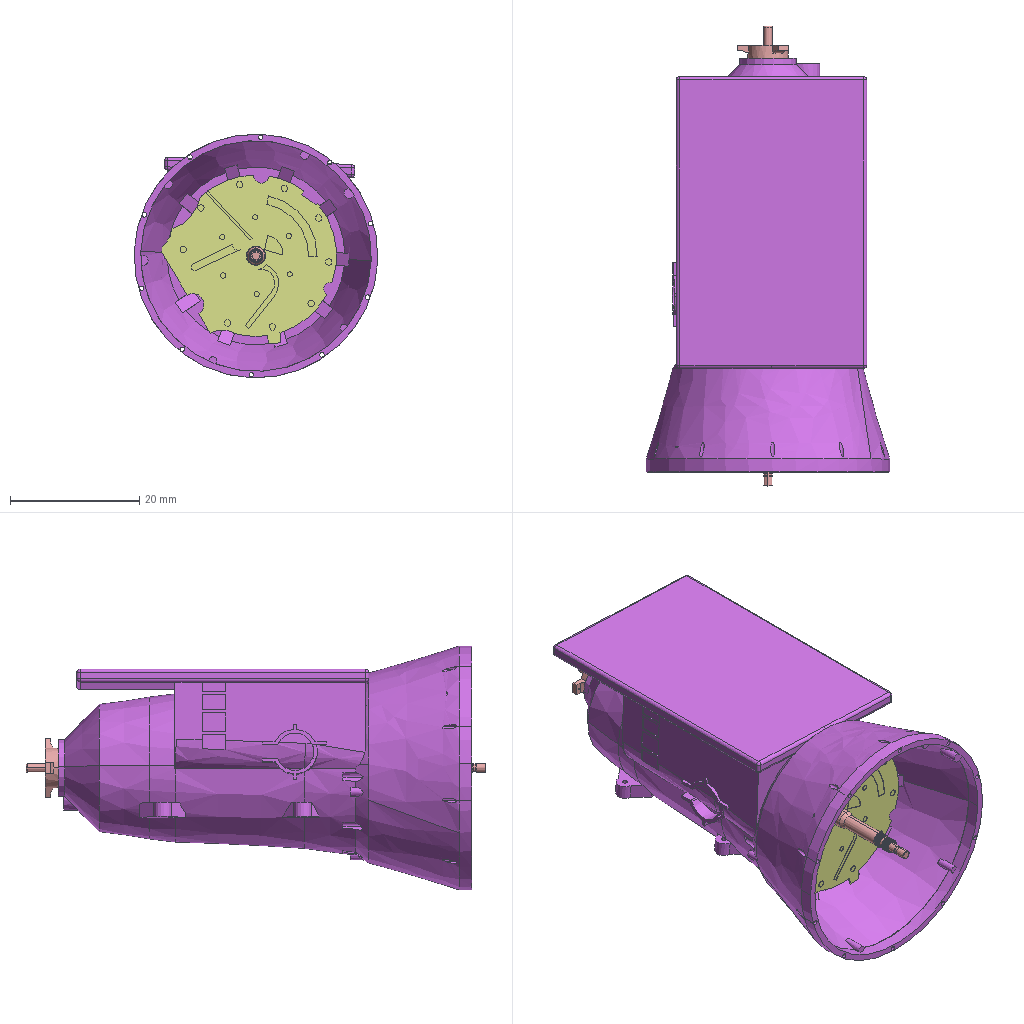Assembly | SolidWorks | 12 different items | 12 placed | box 38 x 71 x 38 mm
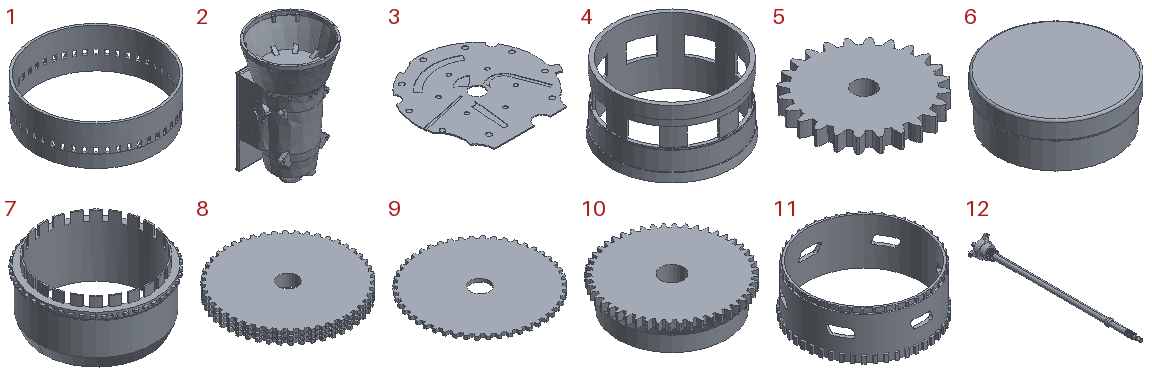Parts list (item | quantity | size | volume | features):
1 | x1 | 18.7 x 18.7 x 6 mm | 97.096 mm3 | features ICE 3, CirPattern 1, Extrusion 1
2 | x1 | 37.751 x 37.751 x 64.09 mm | 13251 mm3 | features ICE 18, Blend 7, DelFace 4, Fillet 4, CirPattern 2, MirrorPattern 2, BlendCut 1, Extrusion 1, Rib 1, Shell 1
3 | x1 | 26.026 x 24.754 x 0.2 mm | 92.065 mm3 | features ICE 4, Extrusion 1
4 | x1 | 19.3 x 19.3 x 10.5 mm | 297.419 mm3 | features ICE 7, Blend 1, CirPattern 1
5 | x1 | 16.941 x 16.941 x 3.8 mm | 406.625 mm3 | features ICE 2, Blend 1, CirPattern 1, Cut 1, Extrusion 1, Fillet 1
6 | x1 | 18 x 18 x 6.8 mm | 1583 mm3 | features Cut 1, Extrusion 1, Fillet 1, ICE 1
7 | x1 | 19.179 x 19.179 x 9.6 mm | 364.987 mm3 | features ICE 5, CirPattern 2, Blend 1, Extrusion 1, Fillet 1
8 | x1 | 19.259 x 19.259 x 1.9 mm | 502.853 mm3 | features ICE 7, CirPattern 3, Cut 1, Extrusion 1
9 | x1 | 19.259 x 19.259 x 0.5 mm | 134.631 mm3 | features CirPattern 1, Cut 1, Extrusion 1, ICE 1
10 | x1 | 16.296 x 16.296 x 4 mm | 653.065 mm3 | features ICE 2, Blend 1, CirPattern 1, Cut 1, Extrusion 1
11 | x1 | 18.565 x 18.565 x 7 mm | 181.204 mm3 | features ICE 4, CirPattern 3, Extrusion 1
12 | x1 | 7.952 x 71.26 x 9.182 mm | 329.036 mm3 | features ICE 5, CirPattern 4, Fillet 3, Cut 2, Revolution 2
Mates (type | each side: item.copy, entity, surface, feature):
Concentric | 12.1 face cylinder Revolve2 | 5.1 face cylinder Cut-Extrude1
Coincident | 12.1 face plane Boss-Extrude3 | 5.1 face plane Boss-Extrude3
Concentric | 12.1 face cylinder Revolve2 | 6.1 face cylinder Cut-Extrude1
Concentric | 12.1 face cylinder Revolve2 | 7.1 face cylinder Cut-Extrude2
Coincident | 6.1 face plane Boss-Extrude2 | 7.1 face plane Loft1
Concentric | 12.1 face cylinder Revolve2 | 8.1 face cylinder Cut-Extrude1
Coincident | 7.1 face plane CirPattern2 | 8.1 face plane Boss-Extrude7
Concentric | 12.1 face cylinder Revolve2 | 9.1 face cylinder Cut-Extrude1
Coincident | 8.1 face plane Boss-Extrude1 | 9.1 face plane Boss-Extrude1
Concentric | 12.1 face cylinder Revolve2 | 10.1 face cylinder Cut-Extrude1
Coincident | 9.1 face plane Boss-Extrude1 | 10.1 face plane Boss-Extrude2
Concentric | 12.1 face cylinder Revolve2 | 11.1 face cylinder Cut-Extrude1
Coincident | 10.1 face plane Boss-Extrude1 | 11.1 face plane Boss-Extrude1
Concentric | 12.1 face cylinder Revolve2 | 1.1 face cylinder Cut-Extrude1
Coincident | 11.1 face plane CirPattern2 | 1.1 face plane Cut-Extrude2 | 2 times
Concentric | 12.1 face cylinder Revolve2 | 4.1 face cylinder Cut-Extrude1
Coincident | 4.1 face plane Loft2 | 1.1 face plane Boss-Extrude2
Concentric | 12.1 face cylinder Revolve2 | 3.1 face cylinder Cut-Extrude1
Coincident | 12.1 face plane Revolve2 | 3.1 face plane Boss-Extrude2
GearDim | 8.1 face cylinder Boss-Extrude7 | 5.1 face cylinder Boss-Extrude1
GearDim | 9.1 face cylinder Boss-Extrude1 | 5.1 face cylinder Boss-Extrude1
GearDim | 10.1 face cylinder Boss-Extrude2 | 5.1 face cylinder Boss-Extrude1
Concentric | 12.1 face cylinder Revolve1 | 2.1 face cylinder Cut-Extrude1
Coincident | 12.1 face plane Revolve1 | 2.1 face plane Boss-Extrude1